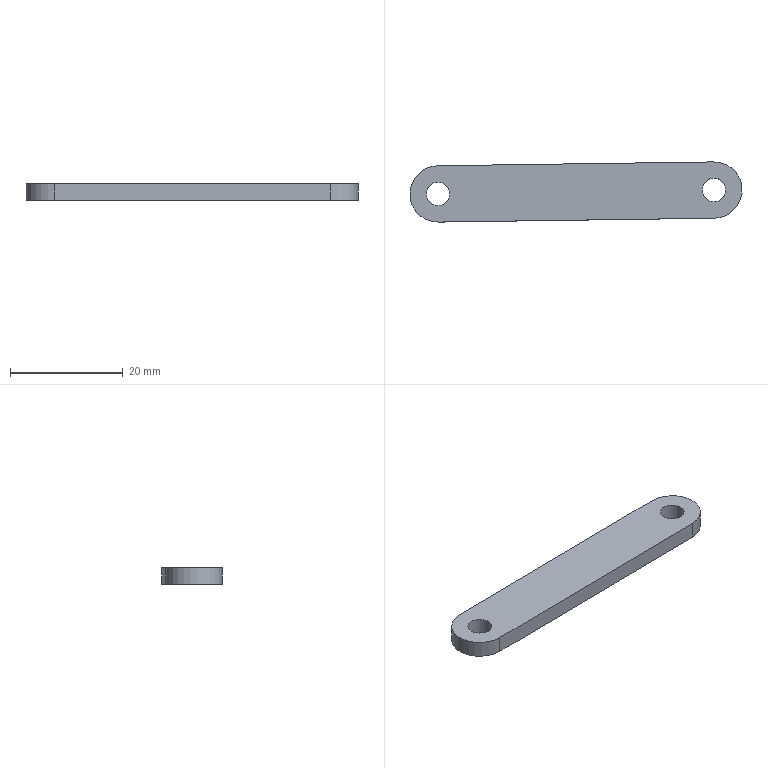Part | NX | features DATUM_CSYS 2, OFFSET_REGION 2, BREP 1, EXTRUDE 1, SCALE 1, SKETCH 1 | 1 solid | 8 faces | box 59.014 x 10.685 x 3 mm | volume 1623 mm3 | cylinder 4 | plane 4 | commonest cylinder face diameters 4.2 x2 10 x2
STEP:
#1=CARTESIAN_POINT('',(91.242,-59.15,-7.5));
#2=VERTEX_POINT('',#1);
#3=CARTESIAN_POINT('',(91.382,-69.149,-7.5));
#4=VERTEX_POINT('',#3);
#5=CARTESIAN_POINT('',(91.312,-64.15,-7.5));
#6=DIRECTION('',(0.,0.,1.));
#7=DIRECTION('',(1.,0.,0.));
#8=AXIS2_PLACEMENT_3D('',#5,#6,#7);
#9=CIRCLE('',#8,5.);
#10=EDGE_CURVE('',#2,#4,#9,.T.);
#11=ORIENTED_EDGE('',*,*,#10,.F.);
#12=CARTESIAN_POINT('',(91.242,-59.15,-10.5));
#13=VERTEX_POINT('',#12);
#14=CARTESIAN_POINT('',(91.242,-59.15,-9.5));
#15=DIRECTION('',(0.,0.,-1.));
#16=VECTOR('',#15,1000.);
#17=LINE('',#14,#16);
#18=EDGE_CURVE('',#2,#13,#17,.T.);
#19=ORIENTED_EDGE('',*,*,#18,.T.);
#20=CARTESIAN_POINT('',(91.382,-69.149,-10.5));
#21=VERTEX_POINT('',#20);
#22=CARTESIAN_POINT('',(91.312,-64.15,-10.5));
#23=DIRECTION('',(0.,0.,1.));
#24=DIRECTION('',(1.,0.,0.));
#25=AXIS2_PLACEMENT_3D('',#22,#23,#24);
#26=CIRCLE('',#25,5.);
#27=EDGE_CURVE('',#13,#21,#26,.T.);
#28=ORIENTED_EDGE('',*,*,#27,.T.);
#29=CARTESIAN_POINT('',(91.382,-69.149,-9.5));
#30=DIRECTION('',(0.,0.,1.));
#31=VECTOR('',#30,1000.);
#32=LINE('',#29,#31);
#33=EDGE_CURVE('',#4,#21,#32,.F.);
#34=ORIENTED_EDGE('',*,*,#33,.F.);
#35=EDGE_LOOP('',(#11,#19,#28,#34));
#36=FACE_BOUND('',#35,.T.);
#37=CARTESIAN_POINT('',(91.312,-64.15,-9.5));
#38=DIRECTION('',(0.,0.,-1.));
#39=DIRECTION('',(-0.9999,-0.01398,0.));
#40=AXIS2_PLACEMENT_3D('',#37,#38,#39);
#41=CYLINDRICAL_SURFACE('',#40,5.);
#42=ADVANCED_FACE('',(#36),#41,.T.);
#43=CARTESIAN_POINT('',(140.256,-58.465,-10.5));
#44=VERTEX_POINT('',#43);
#45=CARTESIAN_POINT('',(91.242,-59.15,-10.5));
#46=DIRECTION('',(0.9999,0.01398,0.));
#47=VECTOR('',#46,1000.);
#48=LINE('',#45,#47);
#49=EDGE_CURVE('',#13,#44,#48,.T.);
#50=ORIENTED_EDGE('',*,*,#49,.F.);
#51=ORIENTED_EDGE('',*,*,#18,.F.);
#52=CARTESIAN_POINT('',(140.256,-58.465,-7.5));
#53=VERTEX_POINT('',#52);
#54=CARTESIAN_POINT('',(91.242,-59.15,-7.5));
#55=DIRECTION('',(0.9999,0.01398,0.));
#56=VECTOR('',#55,1000.);
#57=LINE('',#54,#56);
#58=EDGE_CURVE('',#2,#53,#57,.T.);
#59=ORIENTED_EDGE('',*,*,#58,.T.);
#60=CARTESIAN_POINT('',(140.256,-58.465,-9.5));
#61=DIRECTION('',(0.,0.,1.));
#62=VECTOR('',#61,1000.);
#63=LINE('',#60,#62);
#64=EDGE_CURVE('',#53,#44,#63,.F.);
#65=ORIENTED_EDGE('',*,*,#64,.T.);
#66=EDGE_LOOP('',(#50,#51,#59,#65));
#67=FACE_BOUND('',#66,.T.);
#68=CARTESIAN_POINT('',(91.242,-59.15,-9.5));
#69=DIRECTION('',(-0.01398,0.9999,0.));
#70=DIRECTION('',(-0.9999,-0.01398,0.));
#71=AXIS2_PLACEMENT_3D('',#68,#69,#70);
#72=PLANE('',#71);
#73=ADVANCED_FACE('',(#67),#72,.T.);
#74=CARTESIAN_POINT('',(140.396,-68.464,-10.5));
#75=VERTEX_POINT('',#74);
#76=CARTESIAN_POINT('',(91.382,-69.149,-10.5));
#77=DIRECTION('',(0.9999,0.01398,0.));
#78=VECTOR('',#77,1000.);
#79=LINE('',#76,#78);
#80=EDGE_CURVE('',#21,#75,#79,.T.);
#81=ORIENTED_EDGE('',*,*,#80,.T.);
#82=CARTESIAN_POINT('',(140.396,-68.464,-7.5));
#83=VERTEX_POINT('',#82);
#84=CARTESIAN_POINT('',(140.396,-68.464,-9.5));
#85=DIRECTION('',(0.,0.,-1.));
#86=VECTOR('',#85,1000.);
#87=LINE('',#84,#86);
#88=EDGE_CURVE('',#83,#75,#87,.T.);
#89=ORIENTED_EDGE('',*,*,#88,.F.);
#90=CARTESIAN_POINT('',(91.382,-69.149,-7.5));
#91=DIRECTION('',(0.9999,0.01398,0.));
#92=VECTOR('',#91,1000.);
#93=LINE('',#90,#92);
#94=EDGE_CURVE('',#4,#83,#93,.T.);
#95=ORIENTED_EDGE('',*,*,#94,.F.);
#96=ORIENTED_EDGE('',*,*,#33,.T.);
#97=EDGE_LOOP('',(#81,#89,#95,#96));
#98=FACE_BOUND('',#97,.T.);
#99=CARTESIAN_POINT('',(91.382,-69.149,-9.5));
#100=DIRECTION('',(-0.01398,0.9999,0.));
#101=DIRECTION('',(-0.9999,-0.01398,0.));
#102=AXIS2_PLACEMENT_3D('',#99,#100,#101);
#103=PLANE('',#102);
#104=ADVANCED_FACE('',(#98),#103,.F.);
#105=CARTESIAN_POINT('',(140.326,-63.464,-10.5));
#106=DIRECTION('',(0.,0.,1.));
#107=DIRECTION('',(1.,0.,0.));
#108=AXIS2_PLACEMENT_3D('',#105,#106,#107);
#109=CIRCLE('',#108,5.);
#110=EDGE_CURVE('',#75,#44,#109,.T.);
#111=ORIENTED_EDGE('',*,*,#110,.T.);
#112=ORIENTED_EDGE('',*,*,#64,.F.);
#113=CARTESIAN_POINT('',(140.326,-63.464,-7.5));
#114=DIRECTION('',(0.,0.,1.));
#115=DIRECTION('',(1.,0.,0.));
#116=AXIS2_PLACEMENT_3D('',#113,#114,#115);
#117=CIRCLE('',#116,5.);
#118=EDGE_CURVE('',#83,#53,#117,.T.);
#119=ORIENTED_EDGE('',*,*,#118,.F.);
#120=ORIENTED_EDGE('',*,*,#88,.T.);
#121=EDGE_LOOP('',(#111,#112,#119,#120));
#122=FACE_BOUND('',#121,.T.);
#123=CARTESIAN_POINT('',(140.326,-63.464,-9.5));
#124=DIRECTION('',(0.,0.,-1.));
#125=DIRECTION('',(-0.9999,-0.01398,0.));
#126=AXIS2_PLACEMENT_3D('',#123,#124,#125);
#127=CYLINDRICAL_SURFACE('',#126,5.);
#128=ADVANCED_FACE('',(#122),#127,.T.);
#129=CARTESIAN_POINT('',(142.426,-63.464,-7.5));
#130=VERTEX_POINT('',#129);
#131=CARTESIAN_POINT('',(140.326,-63.464,-7.5));
#132=DIRECTION('',(0.,0.,1.));
#133=DIRECTION('',(1.,0.,0.));
#134=AXIS2_PLACEMENT_3D('',#131,#132,#133);
#135=CIRCLE('',#134,2.1);
#136=EDGE_CURVE('',#130,#130,#135,.F.);
#137=ORIENTED_EDGE('',*,*,#136,.T.);
#138=EDGE_LOOP('',(#137));
#139=FACE_BOUND('',#138,.T.);
#140=CARTESIAN_POINT('',(93.412,-64.15,-7.5));
#141=VERTEX_POINT('',#140);
#142=CARTESIAN_POINT('',(91.312,-64.15,-7.5));
#143=DIRECTION('',(0.,0.,1.));
#144=DIRECTION('',(1.,0.,0.));
#145=AXIS2_PLACEMENT_3D('',#142,#143,#144);
#146=CIRCLE('',#145,2.1);
#147=EDGE_CURVE('',#141,#141,#146,.F.);
#148=ORIENTED_EDGE('',*,*,#147,.T.);
#149=EDGE_LOOP('',(#148));
#150=FACE_BOUND('',#149,.T.);
#151=ORIENTED_EDGE('',*,*,#58,.F.);
#152=ORIENTED_EDGE('',*,*,#10,.T.);
#153=ORIENTED_EDGE('',*,*,#94,.T.);
#154=ORIENTED_EDGE('',*,*,#118,.T.);
#155=EDGE_LOOP('',(#151,#152,#153,#154));
#156=FACE_BOUND('',#155,.T.);
#157=CARTESIAN_POINT('',(140.326,-63.464,-7.5));
#158=DIRECTION('',(0.,0.,1.));
#159=DIRECTION('',(0.9999,0.01398,0.));
#160=AXIS2_PLACEMENT_3D('',#157,#158,#159);
#161=PLANE('',#160);
#162=ADVANCED_FACE('',(#139,#150,#156),#161,.T.);
#163=CARTESIAN_POINT('',(142.426,-63.464,-10.5));
#164=VERTEX_POINT('',#163);
#165=CARTESIAN_POINT('',(140.326,-63.464,-10.5));
#166=DIRECTION('',(0.,0.,1.));
#167=DIRECTION('',(1.,0.,0.));
#168=AXIS2_PLACEMENT_3D('',#165,#166,#167);
#169=CIRCLE('',#168,2.1);
#170=EDGE_CURVE('',#164,#164,#169,.F.);
#171=ORIENTED_EDGE('',*,*,#170,.F.);
#172=EDGE_LOOP('',(#171));
#173=FACE_BOUND('',#172,.T.);
#174=CARTESIAN_POINT('',(93.412,-64.15,-10.5));
#175=VERTEX_POINT('',#174);
#176=CARTESIAN_POINT('',(91.312,-64.15,-10.5));
#177=DIRECTION('',(0.,0.,1.));
#178=DIRECTION('',(1.,0.,0.));
#179=AXIS2_PLACEMENT_3D('',#176,#177,#178);
#180=CIRCLE('',#179,2.1);
#181=EDGE_CURVE('',#175,#175,#180,.F.);
#182=ORIENTED_EDGE('',*,*,#181,.F.);
#183=EDGE_LOOP('',(#182));
#184=FACE_BOUND('',#183,.T.);
#185=ORIENTED_EDGE('',*,*,#49,.T.);
#186=ORIENTED_EDGE('',*,*,#110,.F.);
#187=ORIENTED_EDGE('',*,*,#80,.F.);
#188=ORIENTED_EDGE('',*,*,#27,.F.);
#189=EDGE_LOOP('',(#185,#186,#187,#188));
#190=FACE_BOUND('',#189,.T.);
#191=CARTESIAN_POINT('',(140.326,-63.464,-10.5));
#192=DIRECTION('',(0.,0.,1.));
#193=DIRECTION('',(0.9999,0.01398,0.));
#194=AXIS2_PLACEMENT_3D('',#191,#192,#193);
#195=PLANE('',#194);
#196=ADVANCED_FACE('',(#173,#184,#190),#195,.F.);
#197=ORIENTED_EDGE('',*,*,#147,.F.);
#198=EDGE_LOOP('',(#197));
#199=FACE_BOUND('',#198,.T.);
#200=ORIENTED_EDGE('',*,*,#181,.T.);
#201=EDGE_LOOP('',(#200));
#202=FACE_BOUND('',#201,.T.);
#203=CARTESIAN_POINT('',(91.312,-64.15,-4.5));
#204=DIRECTION('',(0.,0.,-1.));
#205=DIRECTION('',(-1.,0.,0.));
#206=AXIS2_PLACEMENT_3D('',#203,#204,#205);
#207=CYLINDRICAL_SURFACE('',#206,2.1);
#208=ADVANCED_FACE('',(#199,#202),#207,.F.);
#209=ORIENTED_EDGE('',*,*,#136,.F.);
#210=EDGE_LOOP('',(#209));
#211=FACE_BOUND('',#210,.T.);
#212=ORIENTED_EDGE('',*,*,#170,.T.);
#213=EDGE_LOOP('',(#212));
#214=FACE_BOUND('',#213,.T.);
#215=CARTESIAN_POINT('',(140.326,-63.464,-4.5));
#216=DIRECTION('',(0.,0.,-1.));
#217=DIRECTION('',(-1.,0.,0.));
#218=AXIS2_PLACEMENT_3D('',#215,#216,#217);
#219=CYLINDRICAL_SURFACE('',#218,2.1);
#220=ADVANCED_FACE('',(#211,#214),#219,.F.);
#221=CLOSED_SHELL('',(#42,#73,#104,#128,#162,#196,#208,#220));
#222=MANIFOLD_SOLID_BREP('',#221);
#223=(LENGTH_UNIT()NAMED_UNIT(*)SI_UNIT(.MILLI.,.METRE.));
#224=UNCERTAINTY_MEASURE_WITH_UNIT(LENGTH_MEASURE(0.00001),#223,'','');
#225=(NAMED_UNIT(*)PLANE_ANGLE_UNIT()SI_UNIT($,.RADIAN.));
#226=(NAMED_UNIT(*)SI_UNIT($,.STERADIAN.)SOLID_ANGLE_UNIT());
#227=(GEOMETRIC_REPRESENTATION_CONTEXT(3)GLOBAL_UNCERTAINTY_ASSIGNED_CONTEXT((#224))GLOBAL_UNIT_ASSIGNED_CONTEXT((#223,#225,#226))REPRESENTATION_CONTEXT('',''));
#228=ADVANCED_BREP_SHAPE_REPRESENTATION('',(#222),#227);